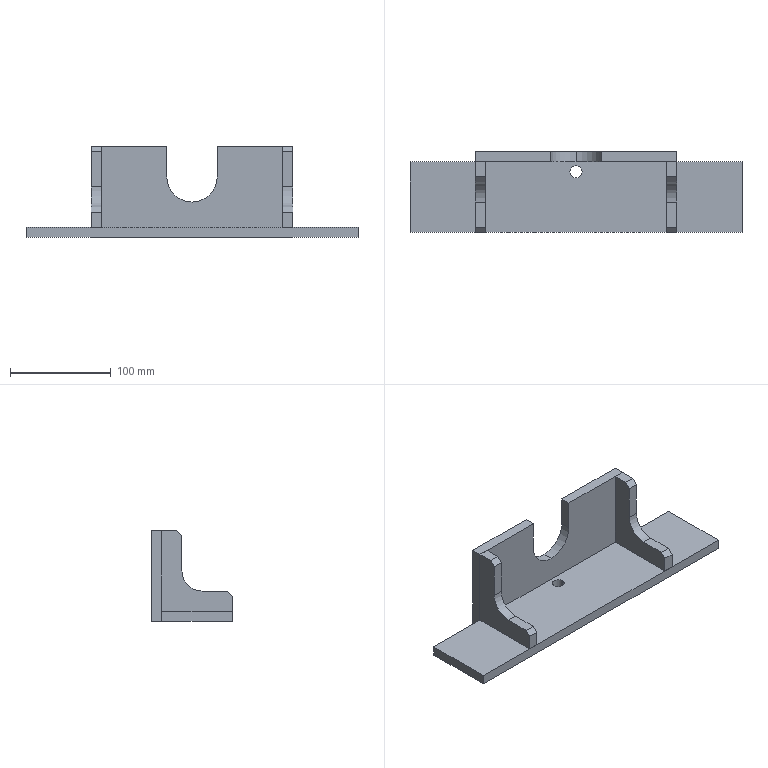Part | STEP file | 4 solids | 41 faces | box 330 x 80 x 90 mm | volume 438268 mm3 | plane 35 | cylinder 6 | commonest cylinder face diameters 12 x2 40 x2 50 x2